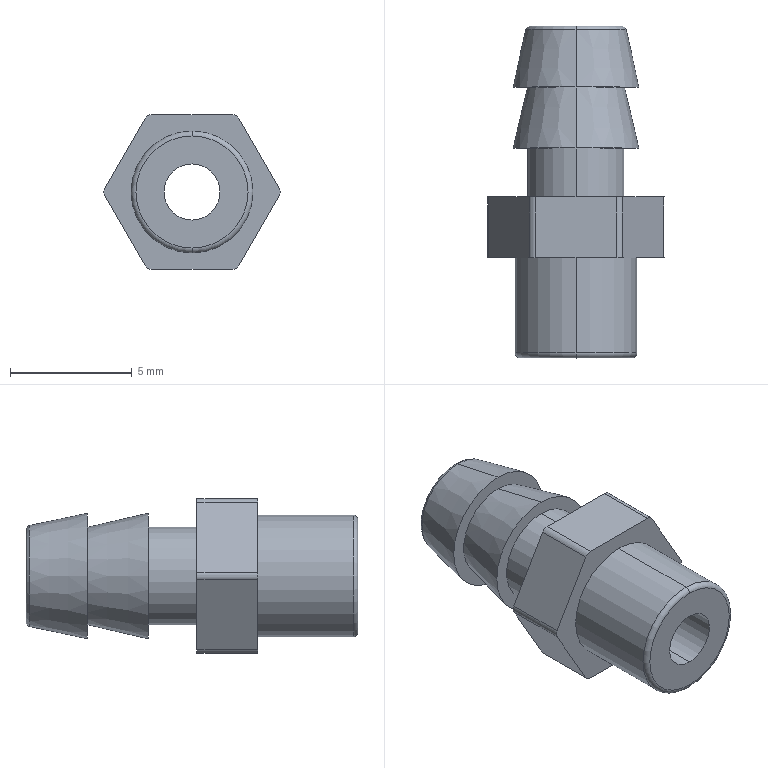Part | SolidWorks | features ICE 5, Fillet 2, Extrusion 1 | 1 solid | 32 faces | box 7.24 x 13.6 x 6.35 mm | volume 219.147 mm3 | cylinder 12 | plane 12 | torus 4 | cone 4 | commonest cylinder face diameters 0.6 x6 2.3 x2 4 x2 5 x2
STEP:
#1=CARTESIAN_POINT('',(0.,9.342,-2.072));
#2=VERTEX_POINT('',#1);
#3=CARTESIAN_POINT('',(0.,9.342,2.072));
#4=VERTEX_POINT('',#3);
#5=CARTESIAN_POINT('',(0.,9.342,0.));
#6=DIRECTION('',(0.,-1.,0.));
#7=DIRECTION('',(0.,0.,-1.));
#8=AXIS2_PLACEMENT_3D('',#5,#6,#7);
#9=CIRCLE('',#8,2.072);
#10=EDGE_CURVE('',#2,#4,#9,.T.);
#11=ORIENTED_EDGE('',*,*,#10,.F.);
#12=CARTESIAN_POINT('',(0.,9.5,-1.877));
#13=VERTEX_POINT('',#12);
#14=CARTESIAN_POINT('',(0.,9.3,-1.877));
#15=DIRECTION('',(1.,0.,0.));
#16=DIRECTION('',(0.,0.,-1.));
#17=AXIS2_PLACEMENT_3D('',#14,#15,#16);
#18=CIRCLE('',#17,0.2);
#19=EDGE_CURVE('',#2,#13,#18,.T.);
#20=ORIENTED_EDGE('',*,*,#19,.T.);
#21=CARTESIAN_POINT('',(0.,9.5,1.877));
#22=VERTEX_POINT('',#21);
#23=CARTESIAN_POINT('',(0.,9.5,0.));
#24=DIRECTION('',(0.,1.,0.));
#25=DIRECTION('',(0.,0.,1.));
#26=AXIS2_PLACEMENT_3D('',#23,#24,#25);
#27=CIRCLE('',#26,1.877);
#28=EDGE_CURVE('',#22,#13,#27,.T.);
#29=ORIENTED_EDGE('',*,*,#28,.F.);
#30=CARTESIAN_POINT('',(0.,9.3,1.877));
#31=DIRECTION('',(-1.,0.,0.));
#32=DIRECTION('',(0.,0.,1.));
#33=AXIS2_PLACEMENT_3D('',#30,#31,#32);
#34=CIRCLE('',#33,0.2);
#35=EDGE_CURVE('',#4,#22,#34,.T.);
#36=ORIENTED_EDGE('',*,*,#35,.F.);
#37=EDGE_LOOP('',(#11,#20,#29,#36));
#38=FACE_OUTER_BOUND('',#37,.T.);
#39=CARTESIAN_POINT('',(0.,9.3,0.));
#40=DIRECTION('',(0.,1.,0.));
#41=DIRECTION('',(0.,0.,1.));
#42=AXIS2_PLACEMENT_3D('',#39,#40,#41);
#43=TOROIDAL_SURFACE('',#42,1.877,0.2);
#44=ADVANCED_FACE('',(#38),#43,.T.);
#45=CARTESIAN_POINT('',(0.,-3.9,2.5));
#46=VERTEX_POINT('',#45);
#47=CARTESIAN_POINT('',(0.,-3.9,-2.5));
#48=VERTEX_POINT('',#47);
#49=CARTESIAN_POINT('',(0.,-3.9,0.));
#50=DIRECTION('',(0.,1.,0.));
#51=DIRECTION('',(0.,0.,-1.));
#52=AXIS2_PLACEMENT_3D('',#49,#50,#51);
#53=CIRCLE('',#52,2.5);
#54=EDGE_CURVE('',#46,#48,#53,.T.);
#55=ORIENTED_EDGE('',*,*,#54,.F.);
#56=CARTESIAN_POINT('',(0.,-4.1,2.3));
#57=VERTEX_POINT('',#56);
#58=CARTESIAN_POINT('',(0.,-3.9,2.3));
#59=DIRECTION('',(1.,0.,0.));
#60=DIRECTION('',(0.,0.,-1.));
#61=AXIS2_PLACEMENT_3D('',#58,#59,#60);
#62=CIRCLE('',#61,0.2);
#63=EDGE_CURVE('',#46,#57,#62,.T.);
#64=ORIENTED_EDGE('',*,*,#63,.T.);
#65=CARTESIAN_POINT('',(0.,-4.1,-2.3));
#66=VERTEX_POINT('',#65);
#67=CARTESIAN_POINT('',(0.,-4.1,0.));
#68=DIRECTION('',(0.,-1.,0.));
#69=DIRECTION('',(0.,0.,-1.));
#70=AXIS2_PLACEMENT_3D('',#67,#68,#69);
#71=CIRCLE('',#70,2.3);
#72=EDGE_CURVE('',#66,#57,#71,.T.);
#73=ORIENTED_EDGE('',*,*,#72,.F.);
#74=CARTESIAN_POINT('',(0.,-3.9,-2.3));
#75=DIRECTION('',(-1.,0.,0.));
#76=DIRECTION('',(0.,0.,1.));
#77=AXIS2_PLACEMENT_3D('',#74,#75,#76);
#78=CIRCLE('',#77,0.2);
#79=EDGE_CURVE('',#48,#66,#78,.T.);
#80=ORIENTED_EDGE('',*,*,#79,.F.);
#81=EDGE_LOOP('',(#55,#64,#73,#80));
#82=FACE_OUTER_BOUND('',#81,.T.);
#83=CARTESIAN_POINT('',(0.,-3.9,0.));
#84=DIRECTION('',(0.,-1.,0.));
#85=DIRECTION('',(0.,0.,-1.));
#86=AXIS2_PLACEMENT_3D('',#83,#84,#85);
#87=TOROIDAL_SURFACE('',#86,2.3,0.2);
#88=ADVANCED_FACE('',(#82),#87,.T.);
#89=CARTESIAN_POINT('',(0.,-4.1,1.15));
#90=VERTEX_POINT('',#89);
#91=CARTESIAN_POINT('',(0.,-4.1,-1.15));
#92=VERTEX_POINT('',#91);
#93=CARTESIAN_POINT('',(0.,-4.1,0.));
#94=DIRECTION('',(0.,-1.,0.));
#95=DIRECTION('',(0.,0.,-1.));
#96=AXIS2_PLACEMENT_3D('',#93,#94,#95);
#97=CIRCLE('',#96,1.15);
#98=EDGE_CURVE('',#90,#92,#97,.T.);
#99=ORIENTED_EDGE('',*,*,#98,.T.);
#100=CARTESIAN_POINT('',(0.,9.5,-1.15));
#101=VERTEX_POINT('',#100);
#102=CARTESIAN_POINT('',(0.,-4.1,-1.15));
#103=DIRECTION('',(0.,1.,0.));
#104=VECTOR('',#103,1000.);
#105=LINE('',#102,#104);
#106=EDGE_CURVE('',#92,#101,#105,.T.);
#107=ORIENTED_EDGE('',*,*,#106,.T.);
#108=CARTESIAN_POINT('',(0.,9.5,1.15));
#109=VERTEX_POINT('',#108);
#110=CARTESIAN_POINT('',(0.,9.5,0.));
#111=DIRECTION('',(0.,-1.,0.));
#112=DIRECTION('',(0.,0.,-1.));
#113=AXIS2_PLACEMENT_3D('',#110,#111,#112);
#114=CIRCLE('',#113,1.15);
#115=EDGE_CURVE('',#109,#101,#114,.T.);
#116=ORIENTED_EDGE('',*,*,#115,.F.);
#117=CARTESIAN_POINT('',(0.,-4.1,1.15));
#118=DIRECTION('',(0.,1.,0.));
#119=VECTOR('',#118,1000.);
#120=LINE('',#117,#119);
#121=EDGE_CURVE('',#90,#109,#120,.T.);
#122=ORIENTED_EDGE('',*,*,#121,.F.);
#123=EDGE_LOOP('',(#99,#107,#116,#122));
#124=FACE_OUTER_BOUND('',#123,.T.);
#125=CARTESIAN_POINT('',(0.,-4.1,0.));
#126=DIRECTION('',(0.,1.,0.));
#127=DIRECTION('',(0.,0.,1.));
#128=AXIS2_PLACEMENT_3D('',#125,#126,#127);
#129=CYLINDRICAL_SURFACE('',#128,1.15);
#130=ADVANCED_FACE('',(#124),#129,.F.);
#131=ORIENTED_EDGE('',*,*,#54,.T.);
#132=CARTESIAN_POINT('',(0.,0.,-2.5));
#133=VERTEX_POINT('',#132);
#134=CARTESIAN_POINT('',(0.,-4.1,-2.5));
#135=DIRECTION('',(0.,1.,0.));
#136=VECTOR('',#135,1000.);
#137=LINE('',#134,#136);
#138=EDGE_CURVE('',#48,#133,#137,.T.);
#139=ORIENTED_EDGE('',*,*,#138,.T.);
#140=CARTESIAN_POINT('',(0.,0.,2.5));
#141=VERTEX_POINT('',#140);
#142=CARTESIAN_POINT('',(0.,0.,0.));
#143=DIRECTION('',(0.,-1.,0.));
#144=DIRECTION('',(0.,0.,1.));
#145=AXIS2_PLACEMENT_3D('',#142,#143,#144);
#146=CIRCLE('',#145,2.5);
#147=EDGE_CURVE('',#133,#141,#146,.T.);
#148=ORIENTED_EDGE('',*,*,#147,.T.);
#149=CARTESIAN_POINT('',(0.,-4.1,2.5));
#150=DIRECTION('',(0.,1.,0.));
#151=VECTOR('',#150,1000.);
#152=LINE('',#149,#151);
#153=EDGE_CURVE('',#46,#141,#152,.T.);
#154=ORIENTED_EDGE('',*,*,#153,.F.);
#155=EDGE_LOOP('',(#131,#139,#148,#154));
#156=FACE_OUTER_BOUND('',#155,.T.);
#157=CARTESIAN_POINT('',(0.,-4.1,0.));
#158=DIRECTION('',(0.,1.,0.));
#159=DIRECTION('',(0.,0.,1.));
#160=AXIS2_PLACEMENT_3D('',#157,#158,#159);
#161=CYLINDRICAL_SURFACE('',#160,2.5);
#162=ADVANCED_FACE('',(#156),#161,.T.);
#163=CARTESIAN_POINT('',(0.,9.342,0.));
#164=DIRECTION('',(0.,-1.,0.));
#165=DIRECTION('',(0.,0.,-1.));
#166=AXIS2_PLACEMENT_3D('',#163,#164,#165);
#167=CIRCLE('',#166,2.072);
#168=EDGE_CURVE('',#4,#2,#167,.T.);
#169=ORIENTED_EDGE('',*,*,#168,.T.);
#170=CARTESIAN_POINT('',(0.,7.,-2.57));
#171=VERTEX_POINT('',#170);
#172=CARTESIAN_POINT('',(0.,7.,-2.57));
#173=DIRECTION('',(0.,-0.9781,-0.2079));
#174=VECTOR('',#173,1000.);
#175=LINE('',#172,#174);
#176=EDGE_CURVE('',#2,#171,#175,.T.);
#177=ORIENTED_EDGE('',*,*,#176,.T.);
#178=CARTESIAN_POINT('',(0.,7.,2.57));
#179=VERTEX_POINT('',#178);
#180=CARTESIAN_POINT('',(0.,7.,0.));
#181=DIRECTION('',(0.,1.,0.));
#182=DIRECTION('',(0.,0.,1.));
#183=AXIS2_PLACEMENT_3D('',#180,#181,#182);
#184=CIRCLE('',#183,2.57);
#185=EDGE_CURVE('',#171,#179,#184,.T.);
#186=ORIENTED_EDGE('',*,*,#185,.T.);
#187=CARTESIAN_POINT('',(0.,7.,2.57));
#188=DIRECTION('',(0.,-0.9781,0.2079));
#189=VECTOR('',#188,1000.);
#190=LINE('',#187,#189);
#191=EDGE_CURVE('',#4,#179,#190,.T.);
#192=ORIENTED_EDGE('',*,*,#191,.F.);
#193=EDGE_LOOP('',(#169,#177,#186,#192));
#194=FACE_OUTER_BOUND('',#193,.T.);
#195=CARTESIAN_POINT('',(0.,7.,0.));
#196=DIRECTION('',(0.,-1.,0.));
#197=DIRECTION('',(0.,0.,1.));
#198=AXIS2_PLACEMENT_3D('',#195,#196,#197);
#199=CONICAL_SURFACE('',#198,2.57,0.2094);
#200=ADVANCED_FACE('',(#194),#199,.T.);
#201=CARTESIAN_POINT('',(0.,7.,-1.993));
#202=VERTEX_POINT('',#201);
#203=CARTESIAN_POINT('',(0.,7.,1.993));
#204=VERTEX_POINT('',#203);
#205=CARTESIAN_POINT('',(0.,7.,0.));
#206=DIRECTION('',(0.,1.,0.));
#207=DIRECTION('',(0.,0.,1.));
#208=AXIS2_PLACEMENT_3D('',#205,#206,#207);
#209=CIRCLE('',#208,1.993);
#210=EDGE_CURVE('',#202,#204,#209,.T.);
#211=ORIENTED_EDGE('',*,*,#210,.F.);
#212=CARTESIAN_POINT('',(0.,4.5,-2.57));
#213=VERTEX_POINT('',#212);
#214=CARTESIAN_POINT('',(0.,4.5,-2.57));
#215=DIRECTION('',(0.,-0.9744,-0.225));
#216=VECTOR('',#215,1000.);
#217=LINE('',#214,#216);
#218=EDGE_CURVE('',#202,#213,#217,.T.);
#219=ORIENTED_EDGE('',*,*,#218,.T.);
#220=CARTESIAN_POINT('',(0.,4.5,2.57));
#221=VERTEX_POINT('',#220);
#222=CARTESIAN_POINT('',(0.,4.5,0.));
#223=DIRECTION('',(0.,1.,0.));
#224=DIRECTION('',(0.,0.,1.));
#225=AXIS2_PLACEMENT_3D('',#222,#223,#224);
#226=CIRCLE('',#225,2.57);
#227=EDGE_CURVE('',#213,#221,#226,.T.);
#228=ORIENTED_EDGE('',*,*,#227,.T.);
#229=CARTESIAN_POINT('',(0.,4.5,2.57));
#230=DIRECTION('',(0.,-0.9744,0.225));
#231=VECTOR('',#230,1000.);
#232=LINE('',#229,#231);
#233=EDGE_CURVE('',#204,#221,#232,.T.);
#234=ORIENTED_EDGE('',*,*,#233,.F.);
#235=EDGE_LOOP('',(#211,#219,#228,#234));
#236=FACE_OUTER_BOUND('',#235,.T.);
#237=CARTESIAN_POINT('',(0.,4.5,0.));
#238=DIRECTION('',(0.,-1.,0.));
#239=DIRECTION('',(0.,0.,1.));
#240=AXIS2_PLACEMENT_3D('',#237,#238,#239);
#241=CONICAL_SURFACE('',#240,2.57,0.2269);
#242=ADVANCED_FACE('',(#236),#241,.T.);
#243=CARTESIAN_POINT('',(0.,4.5,2.));
#244=VERTEX_POINT('',#243);
#245=CARTESIAN_POINT('',(0.,4.5,-2.));
#246=VERTEX_POINT('',#245);
#247=CARTESIAN_POINT('',(0.,4.5,0.));
#248=DIRECTION('',(0.,1.,0.));
#249=DIRECTION('',(0.,0.,1.));
#250=AXIS2_PLACEMENT_3D('',#247,#248,#249);
#251=CIRCLE('',#250,2.);
#252=EDGE_CURVE('',#244,#246,#251,.T.);
#253=ORIENTED_EDGE('',*,*,#252,.F.);
#254=CARTESIAN_POINT('',(0.,2.5,2.));
#255=VERTEX_POINT('',#254);
#256=CARTESIAN_POINT('',(0.,4.5,2.));
#257=DIRECTION('',(0.,-1.,0.));
#258=VECTOR('',#257,1000.);
#259=LINE('',#256,#258);
#260=EDGE_CURVE('',#244,#255,#259,.T.);
#261=ORIENTED_EDGE('',*,*,#260,.T.);
#262=CARTESIAN_POINT('',(0.,2.5,-2.));
#263=VERTEX_POINT('',#262);
#264=CARTESIAN_POINT('',(0.,2.5,0.));
#265=DIRECTION('',(0.,1.,0.));
#266=DIRECTION('',(0.,0.,1.));
#267=AXIS2_PLACEMENT_3D('',#264,#265,#266);
#268=CIRCLE('',#267,2.);
#269=EDGE_CURVE('',#255,#263,#268,.T.);
#270=ORIENTED_EDGE('',*,*,#269,.T.);
#271=CARTESIAN_POINT('',(0.,4.5,-2.));
#272=DIRECTION('',(0.,-1.,0.));
#273=VECTOR('',#272,1000.);
#274=LINE('',#271,#273);
#275=EDGE_CURVE('',#246,#263,#274,.T.);
#276=ORIENTED_EDGE('',*,*,#275,.F.);
#277=EDGE_LOOP('',(#253,#261,#270,#276));
#278=FACE_OUTER_BOUND('',#277,.T.);
#279=CARTESIAN_POINT('',(0.,4.5,0.));
#280=DIRECTION('',(0.,-1.,0.));
#281=DIRECTION('',(0.,0.,-1.));
#282=AXIS2_PLACEMENT_3D('',#279,#280,#281);
#283=CYLINDRICAL_SURFACE('',#282,2.);
#284=ADVANCED_FACE('',(#278),#283,.T.);
#285=CARTESIAN_POINT('',(1.92,2.5,3.025));
#286=VERTEX_POINT('',#285);
#287=CARTESIAN_POINT('',(3.58,2.5,0.15));
#288=VERTEX_POINT('',#287);
#289=CARTESIAN_POINT('',(1.833,2.5,3.175));
#290=DIRECTION('',(0.5,0.,-0.866));
#291=VECTOR('',#290,1000.);
#292=LINE('',#289,#291);
#293=EDGE_CURVE('',#286,#288,#292,.T.);
#294=ORIENTED_EDGE('',*,*,#293,.F.);
#295=CARTESIAN_POINT('',(1.92,0.,3.025));
#296=VERTEX_POINT('',#295);
#297=CARTESIAN_POINT('',(1.92,2.5,3.025));
#298=DIRECTION('',(0.,-1.,0.));
#299=VECTOR('',#298,1000.);
#300=LINE('',#297,#299);
#301=EDGE_CURVE('',#286,#296,#300,.T.);
#302=ORIENTED_EDGE('',*,*,#301,.T.);
#303=CARTESIAN_POINT('',(3.58,0.,0.15));
#304=VERTEX_POINT('',#303);
#305=CARTESIAN_POINT('',(1.833,0.,3.175));
#306=DIRECTION('',(0.5,0.,-0.866));
#307=VECTOR('',#306,1000.);
#308=LINE('',#305,#307);
#309=EDGE_CURVE('',#296,#304,#308,.T.);
#310=ORIENTED_EDGE('',*,*,#309,.T.);
#311=CARTESIAN_POINT('',(3.58,2.5,0.15));
#312=DIRECTION('',(0.,1.,0.));
#313=VECTOR('',#312,1000.);
#314=LINE('',#311,#313);
#315=EDGE_CURVE('',#304,#288,#314,.T.);
#316=ORIENTED_EDGE('',*,*,#315,.T.);
#317=EDGE_LOOP('',(#294,#302,#310,#316));
#318=FACE_OUTER_BOUND('',#317,.T.);
#319=CARTESIAN_POINT('',(1.833,2.5,3.175));
#320=DIRECTION('',(-0.866,0.,-0.5));
#321=DIRECTION('',(-0.5,0.,0.866));
#322=AXIS2_PLACEMENT_3D('',#319,#320,#321);
#323=PLANE('',#322);
#324=ADVANCED_FACE('',(#318),#323,.F.);
#325=CARTESIAN_POINT('',(3.58,2.5,-0.15));
#326=VERTEX_POINT('',#325);
#327=CARTESIAN_POINT('',(1.92,2.5,-3.025));
#328=VERTEX_POINT('',#327);
#329=CARTESIAN_POINT('',(3.666,2.5,0.));
#330=DIRECTION('',(-0.5,0.,-0.866));
#331=VECTOR('',#330,1000.);
#332=LINE('',#329,#331);
#333=EDGE_CURVE('',#326,#328,#332,.T.);
#334=ORIENTED_EDGE('',*,*,#333,.F.);
#335=CARTESIAN_POINT('',(3.58,0.,-0.15));
#336=VERTEX_POINT('',#335);
#337=CARTESIAN_POINT('',(3.58,2.5,-0.15));
#338=DIRECTION('',(0.,-1.,0.));
#339=VECTOR('',#338,1000.);
#340=LINE('',#337,#339);
#341=EDGE_CURVE('',#326,#336,#340,.T.);
#342=ORIENTED_EDGE('',*,*,#341,.T.);
#343=CARTESIAN_POINT('',(1.92,0.,-3.025));
#344=VERTEX_POINT('',#343);
#345=CARTESIAN_POINT('',(3.666,0.,0.));
#346=DIRECTION('',(-0.5,0.,-0.866));
#347=VECTOR('',#346,1000.);
#348=LINE('',#345,#347);
#349=EDGE_CURVE('',#336,#344,#348,.T.);
#350=ORIENTED_EDGE('',*,*,#349,.T.);
#351=CARTESIAN_POINT('',(1.92,2.5,-3.025));
#352=DIRECTION('',(0.,1.,0.));
#353=VECTOR('',#352,1000.);
#354=LINE('',#351,#353);
#355=EDGE_CURVE('',#344,#328,#354,.T.);
#356=ORIENTED_EDGE('',*,*,#355,.T.);
#357=EDGE_LOOP('',(#334,#342,#350,#356));
#358=FACE_OUTER_BOUND('',#357,.T.);
#359=CARTESIAN_POINT('',(3.666,2.5,0.));
#360=DIRECTION('',(-0.866,0.,0.5));
#361=DIRECTION('',(0.5,0.,0.866));
#362=AXIS2_PLACEMENT_3D('',#359,#360,#361);
#363=PLANE('',#362);
#364=ADVANCED_FACE('',(#358),#363,.F.);
#365=CARTESIAN_POINT('',(1.66,0.,-3.175));
#366=VERTEX_POINT('',#365);
#367=CARTESIAN_POINT('',(-1.66,0.,-3.175));
#368=VERTEX_POINT('',#367);
#369=CARTESIAN_POINT('',(1.833,0.,-3.175));
#370=DIRECTION('',(-1.,0.,0.));
#371=VECTOR('',#370,1000.);
#372=LINE('',#369,#371);
#373=EDGE_CURVE('',#366,#368,#372,.T.);
#374=ORIENTED_EDGE('',*,*,#373,.T.);
#375=CARTESIAN_POINT('',(-1.66,2.5,-3.175));
#376=VERTEX_POINT('',#375);
#377=CARTESIAN_POINT('',(-1.66,2.5,-3.175));
#378=DIRECTION('',(0.,1.,0.));
#379=VECTOR('',#378,1000.);
#380=LINE('',#377,#379);
#381=EDGE_CURVE('',#368,#376,#380,.T.);
#382=ORIENTED_EDGE('',*,*,#381,.T.);
#383=CARTESIAN_POINT('',(1.66,2.5,-3.175));
#384=VERTEX_POINT('',#383);
#385=CARTESIAN_POINT('',(1.833,2.5,-3.175));
#386=DIRECTION('',(-1.,0.,0.));
#387=VECTOR('',#386,1000.);
#388=LINE('',#385,#387);
#389=EDGE_CURVE('',#384,#376,#388,.T.);
#390=ORIENTED_EDGE('',*,*,#389,.F.);
#391=CARTESIAN_POINT('',(1.66,2.5,-3.175));
#392=DIRECTION('',(0.,-1.,0.));
#393=VECTOR('',#392,1000.);
#394=LINE('',#391,#393);
#395=EDGE_CURVE('',#384,#366,#394,.T.);
#396=ORIENTED_EDGE('',*,*,#395,.T.);
#397=EDGE_LOOP('',(#374,#382,#390,#396));
#398=FACE_OUTER_BOUND('',#397,.T.);
#399=CARTESIAN_POINT('',(1.833,2.5,-3.175));
#400=DIRECTION('',(0.,0.,1.));
#401=DIRECTION('',(1.,0.,0.));
#402=AXIS2_PLACEMENT_3D('',#399,#400,#401);
#403=PLANE('',#402);
#404=ADVANCED_FACE('',(#398),#403,.F.);
#405=CARTESIAN_POINT('',(-1.92,0.,-3.025));
#406=VERTEX_POINT('',#405);
#407=CARTESIAN_POINT('',(-3.58,0.,-0.15));
#408=VERTEX_POINT('',#407);
#409=CARTESIAN_POINT('',(-1.833,0.,-3.175));
#410=DIRECTION('',(-0.5,0.,0.866));
#411=VECTOR('',#410,1000.);
#412=LINE('',#409,#411);
#413=EDGE_CURVE('',#406,#408,#412,.T.);
#414=ORIENTED_EDGE('',*,*,#413,.T.);
#415=CARTESIAN_POINT('',(-3.58,2.5,-0.15));
#416=VERTEX_POINT('',#415);
#417=CARTESIAN_POINT('',(-3.58,2.5,-0.15));
#418=DIRECTION('',(0.,1.,0.));
#419=VECTOR('',#418,1000.);
#420=LINE('',#417,#419);
#421=EDGE_CURVE('',#408,#416,#420,.T.);
#422=ORIENTED_EDGE('',*,*,#421,.T.);
#423=CARTESIAN_POINT('',(-1.92,2.5,-3.025));
#424=VERTEX_POINT('',#423);
#425=CARTESIAN_POINT('',(-1.833,2.5,-3.175));
#426=DIRECTION('',(-0.5,0.,0.866));
#427=VECTOR('',#426,1000.);
#428=LINE('',#425,#427);
#429=EDGE_CURVE('',#424,#416,#428,.T.);
#430=ORIENTED_EDGE('',*,*,#429,.F.);
#431=CARTESIAN_POINT('',(-1.92,2.5,-3.025));
#432=DIRECTION('',(0.,-1.,0.));
#433=VECTOR('',#432,1000.);
#434=LINE('',#431,#433);
#435=EDGE_CURVE('',#424,#406,#434,.T.);
#436=ORIENTED_EDGE('',*,*,#435,.T.);
#437=EDGE_LOOP('',(#414,#422,#430,#436));
#438=FACE_OUTER_BOUND('',#437,.T.);
#439=CARTESIAN_POINT('',(-1.833,2.5,-3.175));
#440=DIRECTION('',(0.866,0.,0.5));
#441=DIRECTION('',(0.5,0.,-0.866));
#442=AXIS2_PLACEMENT_3D('',#439,#440,#441);
#443=PLANE('',#442);
#444=ADVANCED_FACE('',(#438),#443,.F.);
#445=CARTESIAN_POINT('',(-3.58,0.,0.15));
#446=VERTEX_POINT('',#445);
#447=CARTESIAN_POINT('',(-1.92,0.,3.025));
#448=VERTEX_POINT('',#447);
#449=CARTESIAN_POINT('',(-3.666,0.,0.));
#450=DIRECTION('',(0.5,0.,0.866));
#451=VECTOR('',#450,1000.);
#452=LINE('',#449,#451);
#453=EDGE_CURVE('',#446,#448,#452,.T.);
#454=ORIENTED_EDGE('',*,*,#453,.T.);
#455=CARTESIAN_POINT('',(-1.92,2.5,3.025));
#456=VERTEX_POINT('',#455);
#457=CARTESIAN_POINT('',(-1.92,2.5,3.025));
#458=DIRECTION('',(0.,1.,0.));
#459=VECTOR('',#458,1000.);
#460=LINE('',#457,#459);
#461=EDGE_CURVE('',#448,#456,#460,.T.);
#462=ORIENTED_EDGE('',*,*,#461,.T.);
#463=CARTESIAN_POINT('',(-3.58,2.5,0.15));
#464=VERTEX_POINT('',#463);
#465=CARTESIAN_POINT('',(-3.666,2.5,0.));
#466=DIRECTION('',(0.5,0.,0.866));
#467=VECTOR('',#466,1000.);
#468=LINE('',#465,#467);
#469=EDGE_CURVE('',#464,#456,#468,.T.);
#470=ORIENTED_EDGE('',*,*,#469,.F.);
#471=CARTESIAN_POINT('',(-3.58,2.5,0.15));
#472=DIRECTION('',(0.,-1.,0.));
#473=VECTOR('',#472,1000.);
#474=LINE('',#471,#473);
#475=EDGE_CURVE('',#464,#446,#474,.T.);
#476=ORIENTED_EDGE('',*,*,#475,.T.);
#477=EDGE_LOOP('',(#454,#462,#470,#476));
#478=FACE_OUTER_BOUND('',#477,.T.);
#479=CARTESIAN_POINT('',(-3.666,2.5,0.));
#480=DIRECTION('',(0.866,0.,-0.5));
#481=DIRECTION('',(-0.5,0.,-0.866));
#482=AXIS2_PLACEMENT_3D('',#479,#480,#481);
#483=PLANE('',#482);
#484=ADVANCED_FACE('',(#478),#483,.F.);
#485=CARTESIAN_POINT('',(-1.66,2.5,3.175));
#486=VERTEX_POINT('',#485);
#487=CARTESIAN_POINT('',(1.66,2.5,3.175));
#488=VERTEX_POINT('',#487);
#489=CARTESIAN_POINT('',(-1.833,2.5,3.175));
#490=DIRECTION('',(1.,0.,0.));
#491=VECTOR('',#490,1000.);
#492=LINE('',#489,#491);
#493=EDGE_CURVE('',#486,#488,#492,.T.);
#494=ORIENTED_EDGE('',*,*,#493,.F.);
#495=CARTESIAN_POINT('',(-1.66,0.,3.175));
#496=VERTEX_POINT('',#495);
#497=CARTESIAN_POINT('',(-1.66,2.5,3.175));
#498=DIRECTION('',(0.,-1.,0.));
#499=VECTOR('',#498,1000.);
#500=LINE('',#497,#499);
#501=EDGE_CURVE('',#486,#496,#500,.T.);
#502=ORIENTED_EDGE('',*,*,#501,.T.);
#503=CARTESIAN_POINT('',(1.66,0.,3.175));
#504=VERTEX_POINT('',#503);
#505=CARTESIAN_POINT('',(-1.833,0.,3.175));
#506=DIRECTION('',(1.,0.,0.));
#507=VECTOR('',#506,1000.);
#508=LINE('',#505,#507);
#509=EDGE_CURVE('',#496,#504,#508,.T.);
#510=ORIENTED_EDGE('',*,*,#509,.T.);
#511=CARTESIAN_POINT('',(1.66,2.5,3.175));
#512=DIRECTION('',(0.,1.,0.));
#513=VECTOR('',#512,1000.);
#514=LINE('',#511,#513);
#515=EDGE_CURVE('',#504,#488,#514,.T.);
#516=ORIENTED_EDGE('',*,*,#515,.T.);
#517=EDGE_LOOP('',(#494,#502,#510,#516));
#518=FACE_OUTER_BOUND('',#517,.T.);
#519=CARTESIAN_POINT('',(-1.833,2.5,3.175));
#520=DIRECTION('',(0.,0.,-1.));
#521=DIRECTION('',(-1.,0.,0.));
#522=AXIS2_PLACEMENT_3D('',#519,#520,#521);
#523=PLANE('',#522);
#524=ADVANCED_FACE('',(#518),#523,.F.);
#525=CARTESIAN_POINT('',(0.,2.5,0.));
#526=DIRECTION('',(0.,1.,0.));
#527=DIRECTION('',(0.,0.,1.));
#528=AXIS2_PLACEMENT_3D('',#525,#526,#527);
#529=CIRCLE('',#528,2.);
#530=EDGE_CURVE('',#263,#255,#529,.T.);
#531=ORIENTED_EDGE('',*,*,#530,.F.);
#532=ORIENTED_EDGE('',*,*,#269,.F.);
#533=EDGE_LOOP('',(#531,#532));
#534=FACE_BOUND('',#533,.T.);
#535=ORIENTED_EDGE('',*,*,#469,.T.);
#536=CARTESIAN_POINT('',(-1.66,2.5,2.875));
#537=DIRECTION('',(0.,1.,0.));
#538=DIRECTION('',(0.,0.,1.));
#539=AXIS2_PLACEMENT_3D('',#536,#537,#538);
#540=CIRCLE('',#539,0.3);
#541=EDGE_CURVE('',#456,#486,#540,.T.);
#542=ORIENTED_EDGE('',*,*,#541,.T.);
#543=ORIENTED_EDGE('',*,*,#493,.T.);
#544=CARTESIAN_POINT('',(1.66,2.5,2.875));
#545=DIRECTION('',(0.,1.,0.));
#546=DIRECTION('',(0.,0.,1.));
#547=AXIS2_PLACEMENT_3D('',#544,#545,#546);
#548=CIRCLE('',#547,0.3);
#549=EDGE_CURVE('',#488,#286,#548,.T.);
#550=ORIENTED_EDGE('',*,*,#549,.T.);
#551=ORIENTED_EDGE('',*,*,#293,.T.);
#552=CARTESIAN_POINT('',(3.32,2.5,0.));
#553=DIRECTION('',(0.,1.,0.));
#554=DIRECTION('',(0.,0.,1.));
#555=AXIS2_PLACEMENT_3D('',#552,#553,#554);
#556=CIRCLE('',#555,0.3);
#557=EDGE_CURVE('',#288,#326,#556,.T.);
#558=ORIENTED_EDGE('',*,*,#557,.T.);
#559=ORIENTED_EDGE('',*,*,#333,.T.);
#560=CARTESIAN_POINT('',(1.66,2.5,-2.875));
#561=DIRECTION('',(0.,1.,0.));
#562=DIRECTION('',(0.,0.,1.));
#563=AXIS2_PLACEMENT_3D('',#560,#561,#562);
#564=CIRCLE('',#563,0.3);
#565=EDGE_CURVE('',#328,#384,#564,.T.);
#566=ORIENTED_EDGE('',*,*,#565,.T.);
#567=ORIENTED_EDGE('',*,*,#389,.T.);
#568=CARTESIAN_POINT('',(-1.66,2.5,-2.875));
#569=DIRECTION('',(0.,1.,0.));
#570=DIRECTION('',(0.,0.,1.));
#571=AXIS2_PLACEMENT_3D('',#568,#569,#570);
#572=CIRCLE('',#571,0.3);
#573=EDGE_CURVE('',#376,#424,#572,.T.);
#574=ORIENTED_EDGE('',*,*,#573,.T.);
#575=ORIENTED_EDGE('',*,*,#429,.T.);
#576=CARTESIAN_POINT('',(-3.32,2.5,0.));
#577=DIRECTION('',(0.,1.,0.));
#578=DIRECTION('',(0.,0.,1.));
#579=AXIS2_PLACEMENT_3D('',#576,#577,#578);
#580=CIRCLE('',#579,0.3);
#581=EDGE_CURVE('',#416,#464,#580,.T.);
#582=ORIENTED_EDGE('',*,*,#581,.T.);
#583=EDGE_LOOP('',(#535,#542,#543,#550,#551,#558,#559,#566,#567,#574,#575,#582));
#584=FACE_OUTER_BOUND('',#583,.T.);
#585=CARTESIAN_POINT('',(0.,2.5,0.));
#586=DIRECTION('',(0.,1.,0.));
#587=DIRECTION('',(0.,0.,1.));
#588=AXIS2_PLACEMENT_3D('',#585,#586,#587);
#589=PLANE('',#588);
#590=ADVANCED_FACE('',(#534,#584),#589,.T.);
#591=CARTESIAN_POINT('',(0.,0.,0.));
#592=DIRECTION('',(0.,-1.,0.));
#593=DIRECTION('',(0.,0.,1.));
#594=AXIS2_PLACEMENT_3D('',#591,#592,#593);
#595=CIRCLE('',#594,2.5);
#596=EDGE_CURVE('',#141,#133,#595,.T.);
#597=ORIENTED_EDGE('',*,*,#596,.F.);
#598=ORIENTED_EDGE('',*,*,#147,.F.);
#599=EDGE_LOOP('',(#597,#598));
#600=FACE_BOUND('',#599,.T.);
#601=ORIENTED_EDGE('',*,*,#509,.F.);
#602=CARTESIAN_POINT('',(-1.66,0.,2.875));
#603=DIRECTION('',(0.,-1.,0.));
#604=DIRECTION('',(0.,0.,1.));
#605=AXIS2_PLACEMENT_3D('',#602,#603,#604);
#606=CIRCLE('',#605,0.3);
#607=EDGE_CURVE('',#496,#448,#606,.T.);
#608=ORIENTED_EDGE('',*,*,#607,.T.);
#609=ORIENTED_EDGE('',*,*,#453,.F.);
#610=CARTESIAN_POINT('',(-3.32,0.,0.));
#611=DIRECTION('',(0.,-1.,0.));
#612=DIRECTION('',(0.,0.,1.));
#613=AXIS2_PLACEMENT_3D('',#610,#611,#612);
#614=CIRCLE('',#613,0.3);
#615=EDGE_CURVE('',#446,#408,#614,.T.);
#616=ORIENTED_EDGE('',*,*,#615,.T.);
#617=ORIENTED_EDGE('',*,*,#413,.F.);
#618=CARTESIAN_POINT('',(-1.66,0.,-2.875));
#619=DIRECTION('',(0.,-1.,0.));
#620=DIRECTION('',(0.,0.,1.));
#621=AXIS2_PLACEMENT_3D('',#618,#619,#620);
#622=CIRCLE('',#621,0.3);
#623=EDGE_CURVE('',#406,#368,#622,.T.);
#624=ORIENTED_EDGE('',*,*,#623,.T.);
#625=ORIENTED_EDGE('',*,*,#373,.F.);
#626=CARTESIAN_POINT('',(1.66,0.,-2.875));
#627=DIRECTION('',(0.,-1.,0.));
#628=DIRECTION('',(0.,0.,1.));
#629=AXIS2_PLACEMENT_3D('',#626,#627,#628);
#630=CIRCLE('',#629,0.3);
#631=EDGE_CURVE('',#366,#344,#630,.T.);
#632=ORIENTED_EDGE('',*,*,#631,.T.);
#633=ORIENTED_EDGE('',*,*,#349,.F.);
#634=CARTESIAN_POINT('',(3.32,0.,0.));
#635=DIRECTION('',(0.,-1.,0.));
#636=DIRECTION('',(0.,0.,1.));
#637=AXIS2_PLACEMENT_3D('',#634,#635,#636);
#638=CIRCLE('',#637,0.3);
#639=EDGE_CURVE('',#336,#304,#638,.T.);
#640=ORIENTED_EDGE('',*,*,#639,.T.);
#641=ORIENTED_EDGE('',*,*,#309,.F.);
#642=CARTESIAN_POINT('',(1.66,0.,2.875));
#643=DIRECTION('',(0.,-1.,0.));
#644=DIRECTION('',(0.,0.,1.));
#645=AXIS2_PLACEMENT_3D('',#642,#643,#644);
#646=CIRCLE('',#645,0.3);
#647=EDGE_CURVE('',#296,#504,#646,.T.);
#648=ORIENTED_EDGE('',*,*,#647,.T.);
#649=EDGE_LOOP('',(#601,#608,#609,#616,#617,#624,#625,#632,#633,#640,#641,#648));
#650=FACE_OUTER_BOUND('',#649,.T.);
#651=CARTESIAN_POINT('',(0.,0.,0.));
#652=DIRECTION('',(0.,1.,0.));
#653=DIRECTION('',(0.,0.,1.));
#654=AXIS2_PLACEMENT_3D('',#651,#652,#653);
#655=PLANE('',#654);
#656=ADVANCED_FACE('',(#600,#650),#655,.F.);
#657=ORIENTED_EDGE('',*,*,#260,.F.);
#658=CARTESIAN_POINT('',(0.,4.5,0.));
#659=DIRECTION('',(0.,1.,0.));
#660=DIRECTION('',(0.,0.,1.));
#661=AXIS2_PLACEMENT_3D('',#658,#659,#660);
#662=CIRCLE('',#661,2.);
#663=EDGE_CURVE('',#246,#244,#662,.T.);
#664=ORIENTED_EDGE('',*,*,#663,.F.);
#665=ORIENTED_EDGE('',*,*,#275,.T.);
#666=ORIENTED_EDGE('',*,*,#530,.T.);
#667=EDGE_LOOP('',(#657,#664,#665,#666));
#668=FACE_OUTER_BOUND('',#667,.T.);
#669=CARTESIAN_POINT('',(0.,4.5,0.));
#670=DIRECTION('',(0.,-1.,0.));
#671=DIRECTION('',(0.,0.,-1.));
#672=AXIS2_PLACEMENT_3D('',#669,#670,#671);
#673=CYLINDRICAL_SURFACE('',#672,2.);
#674=ADVANCED_FACE('',(#668),#673,.T.);
#675=ORIENTED_EDGE('',*,*,#218,.F.);
#676=CARTESIAN_POINT('',(0.,7.,0.));
#677=DIRECTION('',(0.,1.,0.));
#678=DIRECTION('',(0.,0.,1.));
#679=AXIS2_PLACEMENT_3D('',#676,#677,#678);
#680=CIRCLE('',#679,1.993);
#681=EDGE_CURVE('',#204,#202,#680,.T.);
#682=ORIENTED_EDGE('',*,*,#681,.F.);
#683=ORIENTED_EDGE('',*,*,#233,.T.);
#684=CARTESIAN_POINT('',(0.,4.5,0.));
#685=DIRECTION('',(0.,1.,0.));
#686=DIRECTION('',(0.,0.,1.));
#687=AXIS2_PLACEMENT_3D('',#684,#685,#686);
#688=CIRCLE('',#687,2.57);
#689=EDGE_CURVE('',#221,#213,#688,.T.);
#690=ORIENTED_EDGE('',*,*,#689,.T.);
#691=EDGE_LOOP('',(#675,#682,#683,#690));
#692=FACE_OUTER_BOUND('',#691,.T.);
#693=CARTESIAN_POINT('',(0.,4.5,0.));
#694=DIRECTION('',(0.,-1.,0.));
#695=DIRECTION('',(0.,0.,1.));
#696=AXIS2_PLACEMENT_3D('',#693,#694,#695);
#697=CONICAL_SURFACE('',#696,2.57,0.2269);
#698=ADVANCED_FACE('',(#692),#697,.T.);
#699=ORIENTED_EDGE('',*,*,#663,.T.);
#700=ORIENTED_EDGE('',*,*,#252,.T.);
#701=EDGE_LOOP('',(#699,#700));
#702=FACE_BOUND('',#701,.T.);
#703=ORIENTED_EDGE('',*,*,#689,.F.);
#704=ORIENTED_EDGE('',*,*,#227,.F.);
#705=EDGE_LOOP('',(#703,#704));
#706=FACE_OUTER_BOUND('',#705,.T.);
#707=CARTESIAN_POINT('',(0.,4.5,0.));
#708=DIRECTION('',(0.,1.,0.));
#709=DIRECTION('',(0.,0.,1.));
#710=AXIS2_PLACEMENT_3D('',#707,#708,#709);
#711=PLANE('',#710);
#712=ADVANCED_FACE('',(#702,#706),#711,.F.);
#713=ORIENTED_EDGE('',*,*,#176,.F.);
#714=ORIENTED_EDGE('',*,*,#10,.T.);
#715=ORIENTED_EDGE('',*,*,#191,.T.);
#716=CARTESIAN_POINT('',(0.,7.,0.));
#717=DIRECTION('',(0.,1.,0.));
#718=DIRECTION('',(0.,0.,1.));
#719=AXIS2_PLACEMENT_3D('',#716,#717,#718);
#720=CIRCLE('',#719,2.57);
#721=EDGE_CURVE('',#179,#171,#720,.T.);
#722=ORIENTED_EDGE('',*,*,#721,.T.);
#723=EDGE_LOOP('',(#713,#714,#715,#722));
#724=FACE_OUTER_BOUND('',#723,.T.);
#725=CARTESIAN_POINT('',(0.,7.,0.));
#726=DIRECTION('',(0.,-1.,0.));
#727=DIRECTION('',(0.,0.,1.));
#728=AXIS2_PLACEMENT_3D('',#725,#726,#727);
#729=CONICAL_SURFACE('',#728,2.57,0.2094);
#730=ADVANCED_FACE('',(#724),#729,.T.);
#731=ORIENTED_EDGE('',*,*,#28,.T.);
#732=CARTESIAN_POINT('',(0.,9.5,0.));
#733=DIRECTION('',(0.,1.,0.));
#734=DIRECTION('',(0.,0.,1.));
#735=AXIS2_PLACEMENT_3D('',#732,#733,#734);
#736=CIRCLE('',#735,1.877);
#737=EDGE_CURVE('',#13,#22,#736,.T.);
#738=ORIENTED_EDGE('',*,*,#737,.T.);
#739=EDGE_LOOP('',(#731,#738));
#740=FACE_OUTER_BOUND('',#739,.T.);
#741=ORIENTED_EDGE('',*,*,#115,.T.);
#742=CARTESIAN_POINT('',(0.,9.5,0.));
#743=DIRECTION('',(0.,-1.,0.));
#744=DIRECTION('',(0.,0.,-1.));
#745=AXIS2_PLACEMENT_3D('',#742,#743,#744);
#746=CIRCLE('',#745,1.15);
#747=EDGE_CURVE('',#101,#109,#746,.T.);
#748=ORIENTED_EDGE('',*,*,#747,.T.);
#749=EDGE_LOOP('',(#741,#748));
#750=FACE_BOUND('',#749,.T.);
#751=CARTESIAN_POINT('',(0.,9.5,0.));
#752=DIRECTION('',(0.,1.,0.));
#753=DIRECTION('',(0.,0.,1.));
#754=AXIS2_PLACEMENT_3D('',#751,#752,#753);
#755=PLANE('',#754);
#756=ADVANCED_FACE('',(#740,#750),#755,.T.);
#757=ORIENTED_EDGE('',*,*,#681,.T.);
#758=ORIENTED_EDGE('',*,*,#210,.T.);
#759=EDGE_LOOP('',(#757,#758));
#760=FACE_BOUND('',#759,.T.);
#761=ORIENTED_EDGE('',*,*,#721,.F.);
#762=ORIENTED_EDGE('',*,*,#185,.F.);
#763=EDGE_LOOP('',(#761,#762));
#764=FACE_OUTER_BOUND('',#763,.T.);
#765=CARTESIAN_POINT('',(0.,7.,0.));
#766=DIRECTION('',(0.,1.,0.));
#767=DIRECTION('',(0.,0.,1.));
#768=AXIS2_PLACEMENT_3D('',#765,#766,#767);
#769=PLANE('',#768);
#770=ADVANCED_FACE('',(#760,#764),#769,.F.);
#771=ORIENTED_EDGE('',*,*,#72,.T.);
#772=CARTESIAN_POINT('',(0.,-4.1,0.));
#773=DIRECTION('',(0.,-1.,0.));
#774=DIRECTION('',(0.,0.,-1.));
#775=AXIS2_PLACEMENT_3D('',#772,#773,#774);
#776=CIRCLE('',#775,2.3);
#777=EDGE_CURVE('',#57,#66,#776,.T.);
#778=ORIENTED_EDGE('',*,*,#777,.T.);
#779=EDGE_LOOP('',(#771,#778));
#780=FACE_OUTER_BOUND('',#779,.T.);
#781=ORIENTED_EDGE('',*,*,#98,.F.);
#782=CARTESIAN_POINT('',(0.,-4.1,0.));
#783=DIRECTION('',(0.,-1.,0.));
#784=DIRECTION('',(0.,0.,-1.));
#785=AXIS2_PLACEMENT_3D('',#782,#783,#784);
#786=CIRCLE('',#785,1.15);
#787=EDGE_CURVE('',#92,#90,#786,.T.);
#788=ORIENTED_EDGE('',*,*,#787,.F.);
#789=EDGE_LOOP('',(#781,#788));
#790=FACE_BOUND('',#789,.T.);
#791=CARTESIAN_POINT('',(0.,-4.1,0.));
#792=DIRECTION('',(0.,-1.,0.));
#793=DIRECTION('',(0.,0.,-1.));
#794=AXIS2_PLACEMENT_3D('',#791,#792,#793);
#795=PLANE('',#794);
#796=ADVANCED_FACE('',(#780,#790),#795,.T.);
#797=ORIENTED_EDGE('',*,*,#138,.F.);
#798=CARTESIAN_POINT('',(0.,-3.9,0.));
#799=DIRECTION('',(0.,1.,0.));
#800=DIRECTION('',(0.,0.,-1.));
#801=AXIS2_PLACEMENT_3D('',#798,#799,#800);
#802=CIRCLE('',#801,2.5);
#803=EDGE_CURVE('',#48,#46,#802,.T.);
#804=ORIENTED_EDGE('',*,*,#803,.T.);
#805=ORIENTED_EDGE('',*,*,#153,.T.);
#806=ORIENTED_EDGE('',*,*,#596,.T.);
#807=EDGE_LOOP('',(#797,#804,#805,#806));
#808=FACE_OUTER_BOUND('',#807,.T.);
#809=CARTESIAN_POINT('',(0.,-4.1,0.));
#810=DIRECTION('',(0.,1.,0.));
#811=DIRECTION('',(0.,0.,1.));
#812=AXIS2_PLACEMENT_3D('',#809,#810,#811);
#813=CYLINDRICAL_SURFACE('',#812,2.5);
#814=ADVANCED_FACE('',(#808),#813,.T.);
#815=ORIENTED_EDGE('',*,*,#106,.F.);
#816=ORIENTED_EDGE('',*,*,#787,.T.);
#817=ORIENTED_EDGE('',*,*,#121,.T.);
#818=ORIENTED_EDGE('',*,*,#747,.F.);
#819=EDGE_LOOP('',(#815,#816,#817,#818));
#820=FACE_OUTER_BOUND('',#819,.T.);
#821=CARTESIAN_POINT('',(0.,-4.1,0.));
#822=DIRECTION('',(0.,1.,0.));
#823=DIRECTION('',(0.,0.,1.));
#824=AXIS2_PLACEMENT_3D('',#821,#822,#823);
#825=CYLINDRICAL_SURFACE('',#824,1.15);
#826=ADVANCED_FACE('',(#820),#825,.F.);
#827=ORIENTED_EDGE('',*,*,#541,.F.);
#828=ORIENTED_EDGE('',*,*,#461,.F.);
#829=ORIENTED_EDGE('',*,*,#607,.F.);
#830=ORIENTED_EDGE('',*,*,#501,.F.);
#831=EDGE_LOOP('',(#827,#828,#829,#830));
#832=FACE_OUTER_BOUND('',#831,.T.);
#833=CARTESIAN_POINT('',(-1.66,2.5,2.875));
#834=DIRECTION('',(0.,-1.,0.));
#835=DIRECTION('',(0.,0.,-1.));
#836=AXIS2_PLACEMENT_3D('',#833,#834,#835);
#837=CYLINDRICAL_SURFACE('',#836,0.3);
#838=ADVANCED_FACE('',(#832),#837,.T.);
#839=ORIENTED_EDGE('',*,*,#581,.F.);
#840=ORIENTED_EDGE('',*,*,#421,.F.);
#841=ORIENTED_EDGE('',*,*,#615,.F.);
#842=ORIENTED_EDGE('',*,*,#475,.F.);
#843=EDGE_LOOP('',(#839,#840,#841,#842));
#844=FACE_OUTER_BOUND('',#843,.T.);
#845=CARTESIAN_POINT('',(-3.32,2.5,0.));
#846=DIRECTION('',(0.,-1.,0.));
#847=DIRECTION('',(0.,0.,-1.));
#848=AXIS2_PLACEMENT_3D('',#845,#846,#847);
#849=CYLINDRICAL_SURFACE('',#848,0.3);
#850=ADVANCED_FACE('',(#844),#849,.T.);
#851=ORIENTED_EDGE('',*,*,#573,.F.);
#852=ORIENTED_EDGE('',*,*,#381,.F.);
#853=ORIENTED_EDGE('',*,*,#623,.F.);
#854=ORIENTED_EDGE('',*,*,#435,.F.);
#855=EDGE_LOOP('',(#851,#852,#853,#854));
#856=FACE_OUTER_BOUND('',#855,.T.);
#857=CARTESIAN_POINT('',(-1.66,2.5,-2.875));
#858=DIRECTION('',(0.,-1.,0.));
#859=DIRECTION('',(0.,0.,-1.));
#860=AXIS2_PLACEMENT_3D('',#857,#858,#859);
#861=CYLINDRICAL_SURFACE('',#860,0.3);
#862=ADVANCED_FACE('',(#856),#861,.T.);
#863=ORIENTED_EDGE('',*,*,#549,.F.);
#864=ORIENTED_EDGE('',*,*,#515,.F.);
#865=ORIENTED_EDGE('',*,*,#647,.F.);
#866=ORIENTED_EDGE('',*,*,#301,.F.);
#867=EDGE_LOOP('',(#863,#864,#865,#866));
#868=FACE_OUTER_BOUND('',#867,.T.);
#869=CARTESIAN_POINT('',(1.66,2.5,2.875));
#870=DIRECTION('',(0.,-1.,0.));
#871=DIRECTION('',(0.,0.,-1.));
#872=AXIS2_PLACEMENT_3D('',#869,#870,#871);
#873=CYLINDRICAL_SURFACE('',#872,0.3);
#874=ADVANCED_FACE('',(#868),#873,.T.);
#875=ORIENTED_EDGE('',*,*,#557,.F.);
#876=ORIENTED_EDGE('',*,*,#315,.F.);
#877=ORIENTED_EDGE('',*,*,#639,.F.);
#878=ORIENTED_EDGE('',*,*,#341,.F.);
#879=EDGE_LOOP('',(#875,#876,#877,#878));
#880=FACE_OUTER_BOUND('',#879,.T.);
#881=CARTESIAN_POINT('',(3.32,2.5,0.));
#882=DIRECTION('',(0.,-1.,0.));
#883=DIRECTION('',(0.,0.,-1.));
#884=AXIS2_PLACEMENT_3D('',#881,#882,#883);
#885=CYLINDRICAL_SURFACE('',#884,0.3);
#886=ADVANCED_FACE('',(#880),#885,.T.);
#887=ORIENTED_EDGE('',*,*,#565,.F.);
#888=ORIENTED_EDGE('',*,*,#355,.F.);
#889=ORIENTED_EDGE('',*,*,#631,.F.);
#890=ORIENTED_EDGE('',*,*,#395,.F.);
#891=EDGE_LOOP('',(#887,#888,#889,#890));
#892=FACE_OUTER_BOUND('',#891,.T.);
#893=CARTESIAN_POINT('',(1.66,2.5,-2.875));
#894=DIRECTION('',(0.,-1.,0.));
#895=DIRECTION('',(0.,0.,-1.));
#896=AXIS2_PLACEMENT_3D('',#893,#894,#895);
#897=CYLINDRICAL_SURFACE('',#896,0.3);
#898=ADVANCED_FACE('',(#892),#897,.T.);
#899=ORIENTED_EDGE('',*,*,#63,.F.);
#900=ORIENTED_EDGE('',*,*,#803,.F.);
#901=ORIENTED_EDGE('',*,*,#79,.T.);
#902=ORIENTED_EDGE('',*,*,#777,.F.);
#903=EDGE_LOOP('',(#899,#900,#901,#902));
#904=FACE_OUTER_BOUND('',#903,.T.);
#905=CARTESIAN_POINT('',(0.,-3.9,0.));
#906=DIRECTION('',(0.,-1.,0.));
#907=DIRECTION('',(0.,0.,-1.));
#908=AXIS2_PLACEMENT_3D('',#905,#906,#907);
#909=TOROIDAL_SURFACE('',#908,2.3,0.2);
#910=ADVANCED_FACE('',(#904),#909,.T.);
#911=ORIENTED_EDGE('',*,*,#19,.F.);
#912=ORIENTED_EDGE('',*,*,#168,.F.);
#913=ORIENTED_EDGE('',*,*,#35,.T.);
#914=ORIENTED_EDGE('',*,*,#737,.F.);
#915=EDGE_LOOP('',(#911,#912,#913,#914));
#916=FACE_OUTER_BOUND('',#915,.T.);
#917=CARTESIAN_POINT('',(0.,9.3,0.));
#918=DIRECTION('',(0.,1.,0.));
#919=DIRECTION('',(0.,0.,1.));
#920=AXIS2_PLACEMENT_3D('',#917,#918,#919);
#921=TOROIDAL_SURFACE('',#920,1.877,0.2);
#922=ADVANCED_FACE('',(#916),#921,.T.);
#923=CLOSED_SHELL('',(#44,#88,#130,#162,#200,#242,#284,#324,#364,#404,#444,#484,#524,#590,#656,#674,#698,#712,#730,#756,#770,#796,#814,#826,#838,#850,#862,#874,#886,#898,#910,#922));
#924=MANIFOLD_SOLID_BREP('',#923);
#925=CARTESIAN_POINT('',(0.,0.,0.));
#926=DIRECTION('',(0.,0.,1.));
#927=DIRECTION('',(1.,0.,0.));
#928=AXIS2_PLACEMENT_3D('',#925,#926,#927);
#929=(LENGTH_UNIT()NAMED_UNIT(*)SI_UNIT(.MILLI.,.METRE.));
#930=UNCERTAINTY_MEASURE_WITH_UNIT(LENGTH_MEASURE(0.00001),#929,'','');
#931=(NAMED_UNIT(*)PLANE_ANGLE_UNIT()SI_UNIT($,.RADIAN.));
#932=(NAMED_UNIT(*)SI_UNIT($,.STERADIAN.)SOLID_ANGLE_UNIT());
#933=(GEOMETRIC_REPRESENTATION_CONTEXT(3)GLOBAL_UNCERTAINTY_ASSIGNED_CONTEXT((#930))GLOBAL_UNIT_ASSIGNED_CONTEXT((#929,#931,#932))REPRESENTATION_CONTEXT('',''));
#934=ADVANCED_BREP_SHAPE_REPRESENTATION('',(#924,#928),#933);